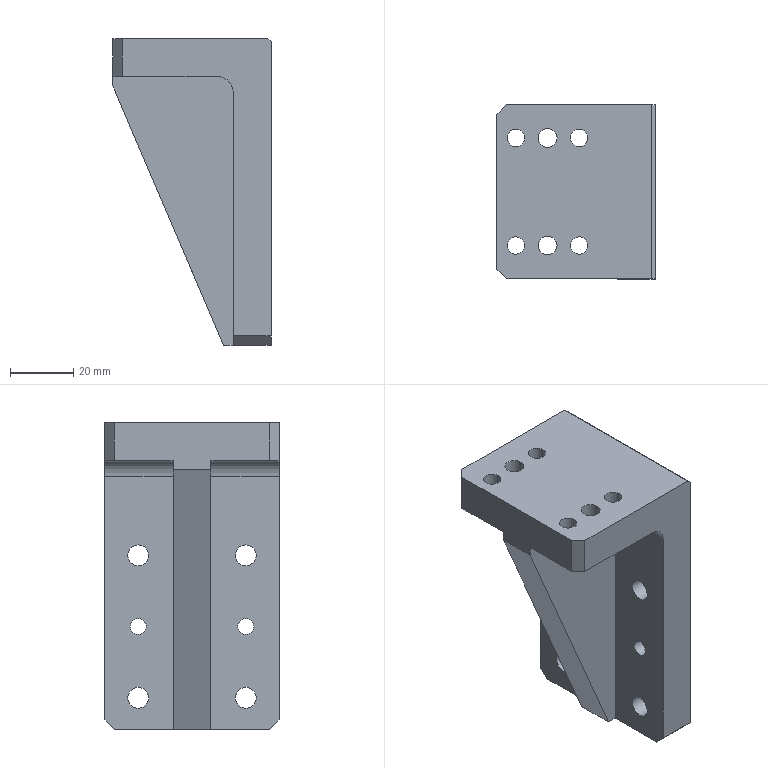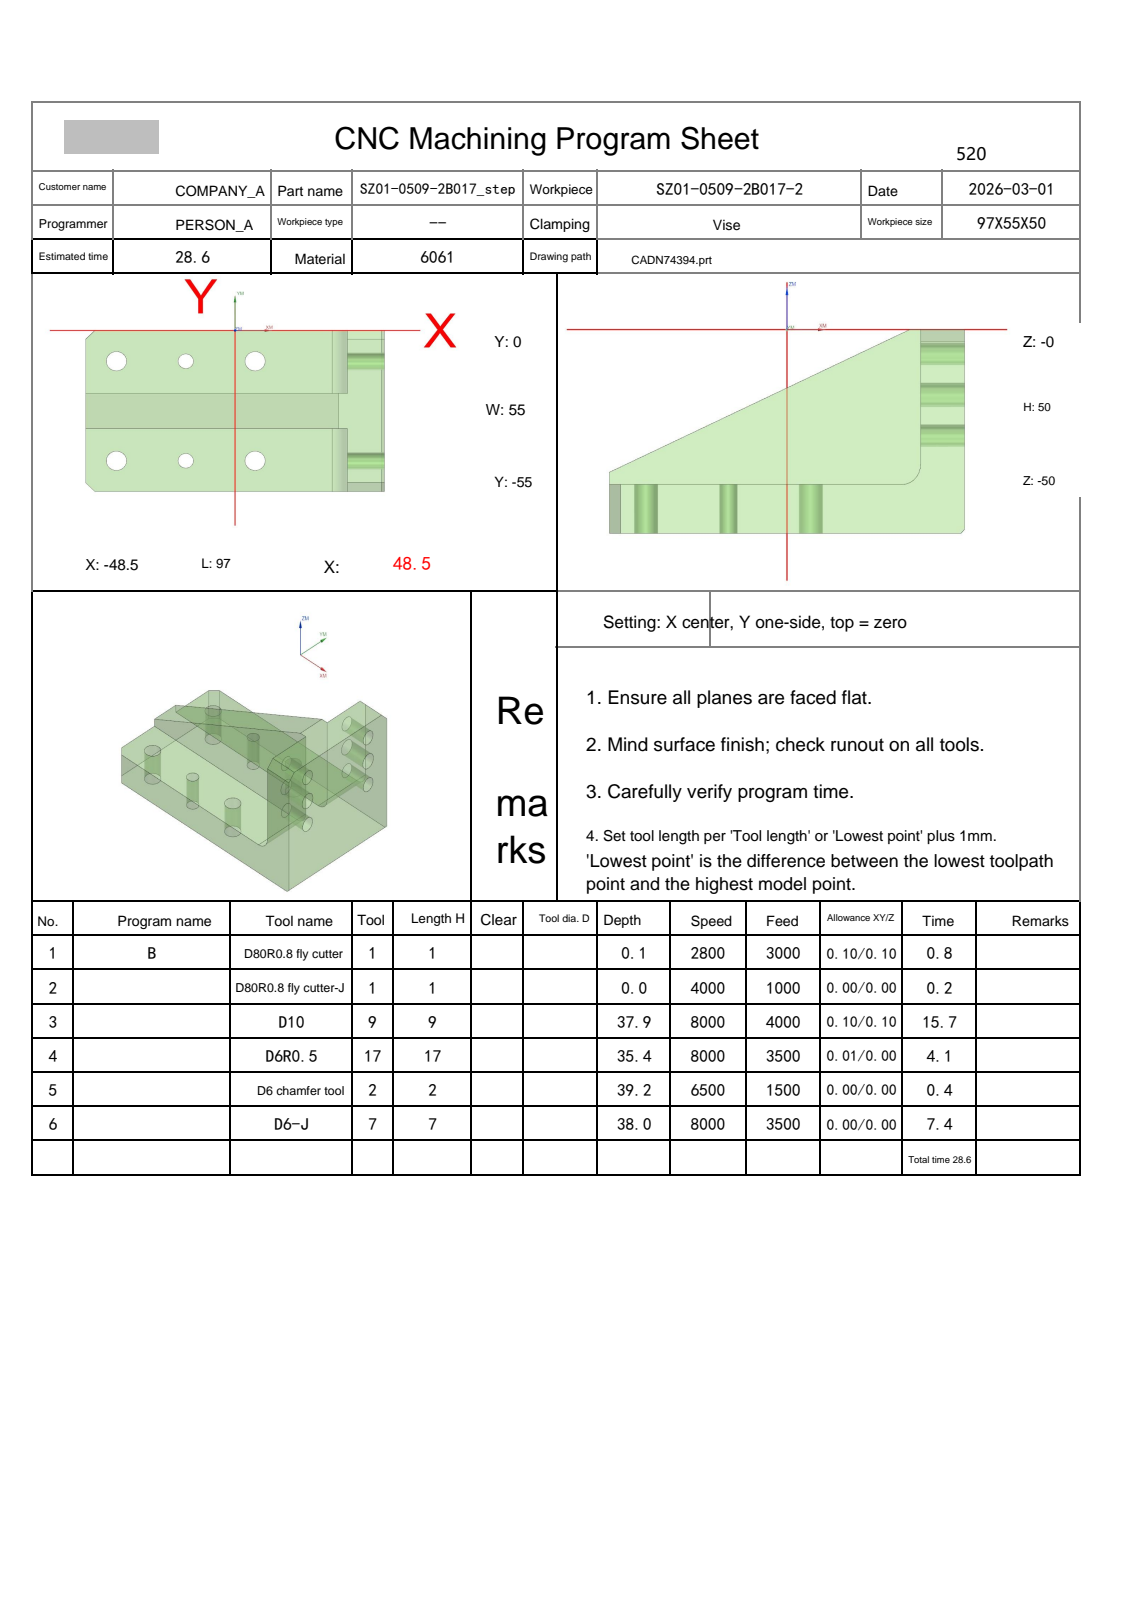NC program | NX | posted by the shop | part box 50 x 55 x 97 mm
Lines 13247 to 13428 of 18128:
N5 T02 M06
(D6 chamfer tool  D=6. R=0. H=02 ce=0.00 di=0.00)
G00 G90 G54 X35.51 Y-52.792 M03 S6500
G43 H02 Z50.
M08
Z.13
G01 Z-1.2 F1500.
G03 X35.585 Y-52.452 I-1.907 J.601
G01 X35.595 Y-52.398
X35.572 Y-52.349
X35.534 Y-52.259
X35.5 Y-52.
Y-34.5
X33.5
X33.241 Y-34.466
X33.151 Y-34.428
Z2.8
G00 Z10.
Y-20.572
Z2.8
G01 Z-1.2
X33.241 Y-20.534
X33.5 Y-20.5
X35.5
Y-3.
X35.534 Y-2.741
X35.572 Y-2.651
X35.595 Y-2.602
X35.585 Y-2.548
G03 X35.51 Y-2.208 I-1.983 J-.261
G01 Z.13
G00 Z10.
X49.49
Z.13
G01 Z-1.2
G03 X49.415 Y-2.548 I1.907 J-.601
G01 X49.405 Y-2.602
X49.428 Y-2.651
X49.466 Y-2.741
X49.5 Y-3.
Y-27.5
Y-52.
X49.466 Y-52.259
X49.428 Y-52.349
X49.405 Y-52.398
X49.415 Y-52.452
G03 X49.49 Y-52.792 I1.983 J.261
G01 Z.13
G00 Z10.
X-49.568 Y-18.472
Z-36.347
G01 Z-39.199
X-49.508 Y-18.386
X-49.5 Y-18.356
Y-3.
X-49.466 Y-2.741
X-49.366 Y-2.5
X-49.207 Y-2.293
X-46.207 Y.707
X-46. Y.866
X-45.759 Y.966
X-45.5 Y1.
X31.5
X31.544 Y.996
X31.58 Y1.021
G03 X31.808 Y1.181 I-.8 J1.386
G01 Z-37.596
G00 Z10.
X4.392 Y-10.096
Z-37.747
G01 Z-39.199
G03 X4.218 Y-10.398 I1.638 J-1.147
G01 X4.192 Y-10.446
X4.2 Y-10.5
G03 X6.5 Y-12.8 I2.3 J0.0
X8.8 Y-10.5 I0.0 J2.3
X6.5 Y-8.2 I-2.3 J0.0
X4.2 Y-10.5 I0.0 J-2.3
G01 X4.192 Y-10.554
X4.218 Y-10.602
G03 X4.392 Y-10.904 I1.813 J.845
G01 Z-37.747
G00 Z10.
X-17.315 Y-10.093
Z-37.716
G01 Z-39.199
G03 X-17.484 Y-10.398 I1.658 J-1.118
G01 X-17.509 Y-10.446
X-17.5 Y-10.5
G03 X-16. Y-12. I1.5 J0.0
X-14.5 Y-10.5 I0.0 J1.5
X-16. Y-9. I-1.5 J0.0
X-17.5 Y-10.5 I0.0 J-1.5
G01 X-17.509 Y-10.554
X-17.484 Y-10.602
G03 X-17.315 Y-10.907 I1.827 J.813
G01 Z-37.716
G00 Z10.
X-40.608 Y-10.096
Z-37.747
G01 Z-39.199
G03 X-40.782 Y-10.398 I1.638 J-1.147
G01 X-40.808 Y-10.446
X-40.8 Y-10.5
G03 X-38.5 Y-12.8 I2.3 J0.0
X-36.2 Y-10.5 I0.0 J2.3
X-38.5 Y-8.2 I-2.3 J0.0
X-40.8 Y-10.5 I0.0 J-2.3
G01 X-40.808 Y-10.554
X-40.782 Y-10.602
G03 X-40.608 Y-10.904 I1.813 J.845
G01 Z-37.747
G00 Z10.
X31.808 Y-56.181
Z-37.596
G01 Z-39.199
G03 X31.58 Y-56.021 I-1.028 J-1.226
G01 X31.544 Y-55.996
X31.5 Y-56.
X-45.5
X-45.759 Y-55.966
X-46. Y-55.866
X-46.207 Y-55.707
X-49.207 Y-52.707
X-49.366 Y-52.5
X-49.466 Y-52.259
X-49.5 Y-52.
Y-36.644
X-49.508 Y-36.614
X-49.568 Y-36.528
Z-36.347
G00 Z-35.449
X-40.608 Y-44.096
Z-37.747
G01 Z-39.199
G03 X-40.782 Y-44.398 I1.638 J-1.147
G01 X-40.808 Y-44.446
X-40.8 Y-44.5
G03 X-38.5 Y-46.8 I2.3 J0.0
X-36.2 Y-44.5 I0.0 J2.3
X-38.5 Y-42.2 I-2.3 J0.0
X-40.8 Y-44.5 I0.0 J-2.3
G01 X-40.808 Y-44.554
X-40.782 Y-44.602
G03 X-40.608 Y-44.904 I1.813 J.845
G01 Z-37.747
G00 Z10.
X-17.315 Y-44.093
Z-37.716
G01 Z-39.199
G03 X-17.484 Y-44.398 I1.658 J-1.118
G01 X-17.509 Y-44.446
X-17.5 Y-44.5
G03 X-16. Y-46. I1.5 J0.0
X-14.5 Y-44.5 I0.0 J1.5
X-16. Y-43. I-1.5 J0.0
X-17.5 Y-44.5 I0.0 J-1.5
G01 X-17.509 Y-44.554
X-17.484 Y-44.602
G03 X-17.315 Y-44.907 I1.827 J.813
G01 Z-37.716
G00 Z10.
X4.392 Y-44.096
Z-37.747
G01 Z-39.199
G03 X4.218 Y-44.398 I1.638 J-1.147
G01 X4.192 Y-44.446
X4.2 Y-44.5
G03 X6.5 Y-46.8 I2.3 J0.0
X8.8 Y-44.5 I0.0 J2.3
X6.5 Y-42.2 I-2.3 J0.0
X4.2 Y-44.5 I0.0 J-2.3
G01 X4.192 Y-44.554
X4.218 Y-44.602
G03 X4.392 Y-44.904 I1.813 J.845
G01 Z-37.747
G00 Z50.
G91 G28 Z0.0
M05
M09
G91 G28 Z0.0
M01